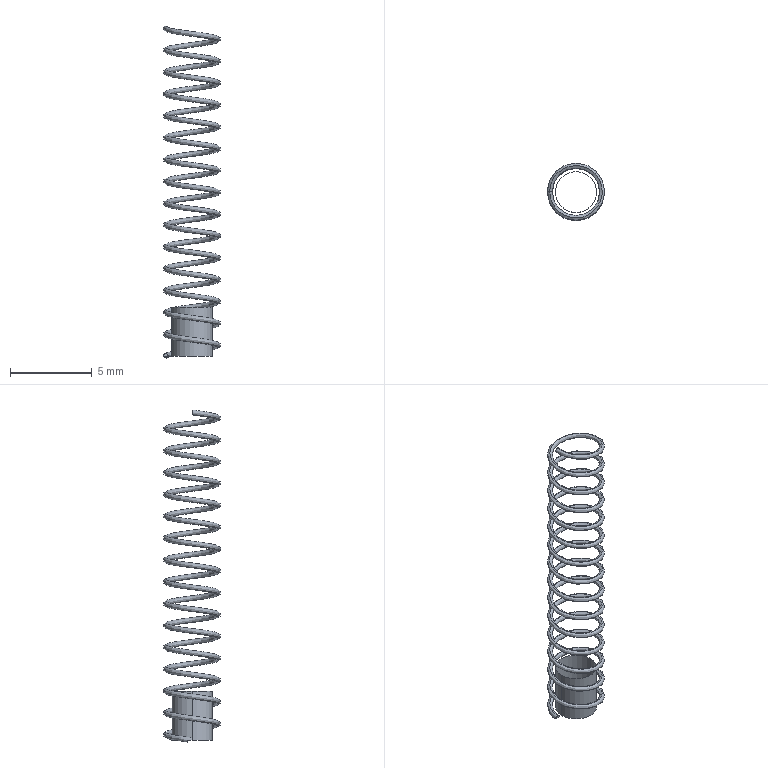Part | NX | features BREP 2 | 1 solid | 9 faces | box 3.5 x 3.5 x 20.261 mm | volume 20.426 mm3 | plane 5 | spline 2 | cylinder 2 | commonest cylinder face diameters 2.5 x2